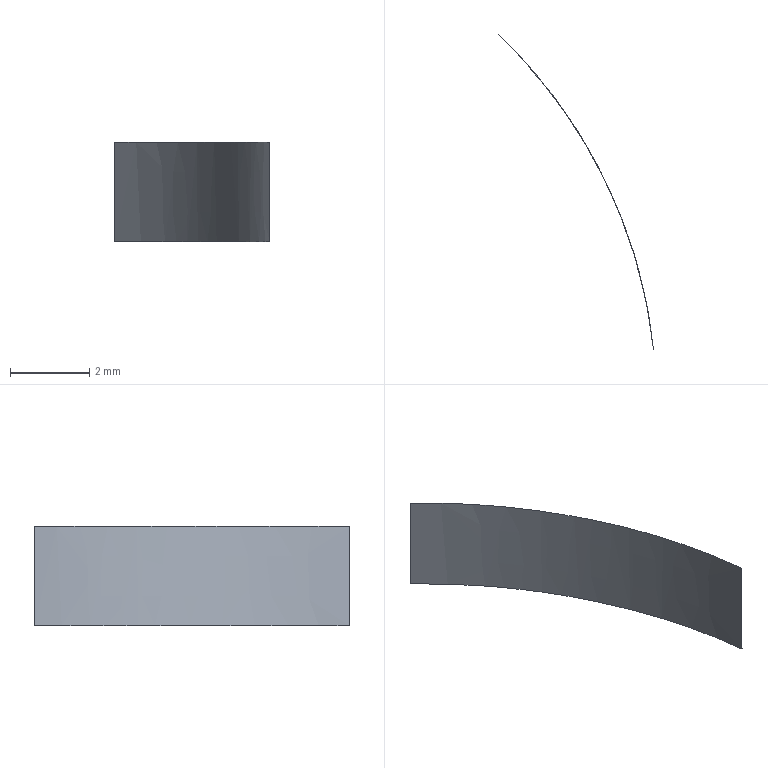Part | STEP file | lll_id366_x_t | 1 solid | 2 faces | box 3.913 x 7.942 x 2.5 mm | volume 0.01666 mm3 | other 1 | cylinder 1 | commonest cylinder face diameters 25.6 x1